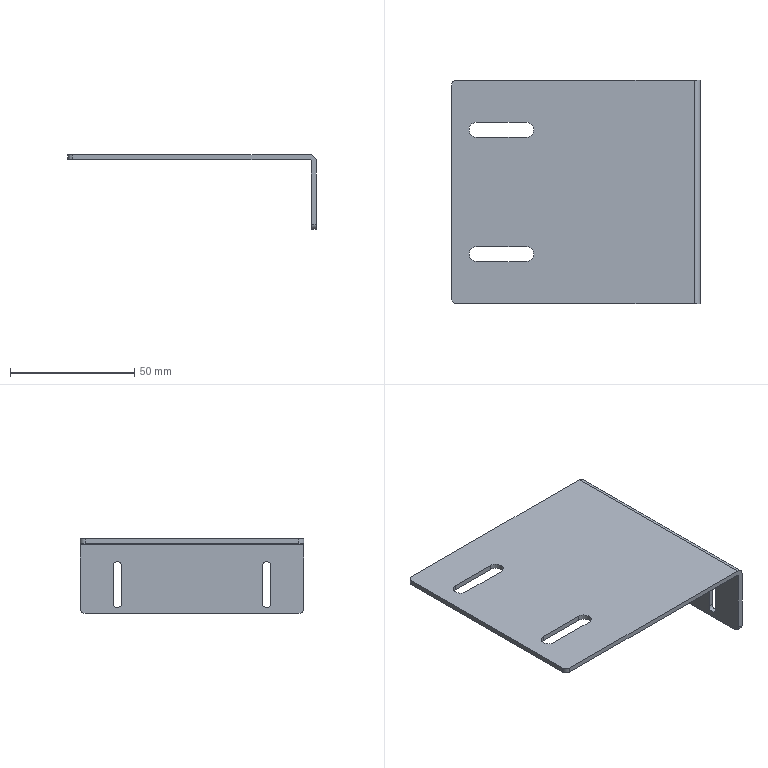Part | SolidWorks | features BaseBody 1 | 1 solid | 34 faces | box 100 x 90 x 30 mm | volume 22076 mm3 | cylinder 18 | plane 16 | commonest cylinder face diameters 3.5 x6 6 x6 4 x4 1 x1 5 x1
STEP:
#1=CARTESIAN_POINT('',(-93.,70.,0.));
#2=VERTEX_POINT('',#1);
#3=CARTESIAN_POINT('',(-90.,73.,0.));
#4=VERTEX_POINT('',#3);
#5=CARTESIAN_POINT('',(-90.,70.,0.));
#6=DIRECTION('',(0.,0.,-1.));
#7=DIRECTION('',(-1.,0.,0.));
#8=AXIS2_PLACEMENT_3D('',#5,#6,#7);
#9=CIRCLE('',#8,3.);
#10=EDGE_CURVE('',#2,#4,#9,.T.);
#11=ORIENTED_EDGE('',*,*,#10,.F.);
#12=CARTESIAN_POINT('',(-93.,70.,-2.));
#13=VERTEX_POINT('',#12);
#14=CARTESIAN_POINT('',(-93.,70.,8.));
#15=DIRECTION('',(0.,0.,-1.));
#16=VECTOR('',#15,1000.);
#17=LINE('',#14,#16);
#18=EDGE_CURVE('',#2,#13,#17,.T.);
#19=ORIENTED_EDGE('',*,*,#18,.T.);
#20=CARTESIAN_POINT('',(-90.,73.,-2.));
#21=VERTEX_POINT('',#20);
#22=CARTESIAN_POINT('',(-90.,70.,-2.));
#23=DIRECTION('',(0.,0.,1.));
#24=DIRECTION('',(-1.,0.,0.));
#25=AXIS2_PLACEMENT_3D('',#22,#23,#24);
#26=CIRCLE('',#25,3.);
#27=EDGE_CURVE('',#21,#13,#26,.T.);
#28=ORIENTED_EDGE('',*,*,#27,.F.);
#29=CARTESIAN_POINT('',(-90.,73.,8.));
#30=DIRECTION('',(0.,0.,1.));
#31=VECTOR('',#30,1000.);
#32=LINE('',#29,#31);
#33=EDGE_CURVE('',#21,#4,#32,.T.);
#34=ORIENTED_EDGE('',*,*,#33,.T.);
#35=EDGE_LOOP('',(#11,#19,#28,#34));
#36=FACE_OUTER_BOUND('',#35,.T.);
#37=CARTESIAN_POINT('',(-90.,70.,8.));
#38=DIRECTION('',(0.,0.,-1.));
#39=DIRECTION('',(-1.,0.,0.));
#40=AXIS2_PLACEMENT_3D('',#37,#38,#39);
#41=CYLINDRICAL_SURFACE('',#40,3.);
#42=ADVANCED_FACE('',(#36),#41,.F.);
#43=CARTESIAN_POINT('',(-93.,20.,0.));
#44=VERTEX_POINT('',#43);
#45=CARTESIAN_POINT('',(-90.,23.,0.));
#46=VERTEX_POINT('',#45);
#47=CARTESIAN_POINT('',(-90.,20.,0.));
#48=DIRECTION('',(0.,0.,-1.));
#49=DIRECTION('',(-1.,0.,0.));
#50=AXIS2_PLACEMENT_3D('',#47,#48,#49);
#51=CIRCLE('',#50,3.);
#52=EDGE_CURVE('',#44,#46,#51,.T.);
#53=ORIENTED_EDGE('',*,*,#52,.F.);
#54=CARTESIAN_POINT('',(-93.,20.,-2.));
#55=VERTEX_POINT('',#54);
#56=CARTESIAN_POINT('',(-93.,20.,8.));
#57=DIRECTION('',(0.,0.,-1.));
#58=VECTOR('',#57,1000.);
#59=LINE('',#56,#58);
#60=EDGE_CURVE('',#44,#55,#59,.T.);
#61=ORIENTED_EDGE('',*,*,#60,.T.);
#62=CARTESIAN_POINT('',(-90.,23.,-2.));
#63=VERTEX_POINT('',#62);
#64=CARTESIAN_POINT('',(-90.,20.,-2.));
#65=DIRECTION('',(0.,0.,1.));
#66=DIRECTION('',(-1.,0.,0.));
#67=AXIS2_PLACEMENT_3D('',#64,#65,#66);
#68=CIRCLE('',#67,3.);
#69=EDGE_CURVE('',#63,#55,#68,.T.);
#70=ORIENTED_EDGE('',*,*,#69,.F.);
#71=CARTESIAN_POINT('',(-90.,23.,8.));
#72=DIRECTION('',(0.,0.,1.));
#73=VECTOR('',#72,1000.);
#74=LINE('',#71,#73);
#75=EDGE_CURVE('',#63,#46,#74,.T.);
#76=ORIENTED_EDGE('',*,*,#75,.T.);
#77=EDGE_LOOP('',(#53,#61,#70,#76));
#78=FACE_OUTER_BOUND('',#77,.T.);
#79=CARTESIAN_POINT('',(-90.,20.,8.));
#80=DIRECTION('',(0.,0.,-1.));
#81=DIRECTION('',(-1.,0.,0.));
#82=AXIS2_PLACEMENT_3D('',#79,#80,#81);
#83=CYLINDRICAL_SURFACE('',#82,3.);
#84=ADVANCED_FACE('',(#78),#83,.F.);
#85=CARTESIAN_POINT('',(0.,75.,-9.25));
#86=VERTEX_POINT('',#85);
#87=CARTESIAN_POINT('',(0.,76.75,-11.));
#88=VERTEX_POINT('',#87);
#89=CARTESIAN_POINT('',(0.,75.,-11.));
#90=DIRECTION('',(-1.,0.,0.));
#91=DIRECTION('',(0.,0.,1.));
#92=AXIS2_PLACEMENT_3D('',#89,#90,#91);
#93=CIRCLE('',#92,1.75);
#94=EDGE_CURVE('',#86,#88,#93,.T.);
#95=ORIENTED_EDGE('',*,*,#94,.F.);
#96=CARTESIAN_POINT('',(-2.,75.,-9.25));
#97=VERTEX_POINT('',#96);
#98=CARTESIAN_POINT('',(8.,75.,-9.25));
#99=DIRECTION('',(-1.,0.,0.));
#100=VECTOR('',#99,1000.);
#101=LINE('',#98,#100);
#102=EDGE_CURVE('',#86,#97,#101,.T.);
#103=ORIENTED_EDGE('',*,*,#102,.T.);
#104=CARTESIAN_POINT('',(-2.,76.75,-11.));
#105=VERTEX_POINT('',#104);
#106=CARTESIAN_POINT('',(-2.,75.,-11.));
#107=DIRECTION('',(1.,0.,0.));
#108=DIRECTION('',(0.,0.,1.));
#109=AXIS2_PLACEMENT_3D('',#106,#107,#108);
#110=CIRCLE('',#109,1.75);
#111=EDGE_CURVE('',#105,#97,#110,.T.);
#112=ORIENTED_EDGE('',*,*,#111,.F.);
#113=CARTESIAN_POINT('',(8.,76.75,-11.));
#114=DIRECTION('',(1.,0.,0.));
#115=VECTOR('',#114,1000.);
#116=LINE('',#113,#115);
#117=EDGE_CURVE('',#105,#88,#116,.T.);
#118=ORIENTED_EDGE('',*,*,#117,.T.);
#119=EDGE_LOOP('',(#95,#103,#112,#118));
#120=FACE_OUTER_BOUND('',#119,.T.);
#121=CARTESIAN_POINT('',(8.,75.,-11.));
#122=DIRECTION('',(-1.,0.,0.));
#123=DIRECTION('',(0.,0.,1.));
#124=AXIS2_PLACEMENT_3D('',#121,#122,#123);
#125=CYLINDRICAL_SURFACE('',#124,1.75);
#126=ADVANCED_FACE('',(#120),#125,.F.);
#127=CARTESIAN_POINT('',(0.,15.,-9.25));
#128=VERTEX_POINT('',#127);
#129=CARTESIAN_POINT('',(0.,16.75,-11.));
#130=VERTEX_POINT('',#129);
#131=CARTESIAN_POINT('',(0.,15.,-11.));
#132=DIRECTION('',(-1.,0.,0.));
#133=DIRECTION('',(0.,0.,1.));
#134=AXIS2_PLACEMENT_3D('',#131,#132,#133);
#135=CIRCLE('',#134,1.75);
#136=EDGE_CURVE('',#128,#130,#135,.T.);
#137=ORIENTED_EDGE('',*,*,#136,.F.);
#138=CARTESIAN_POINT('',(-2.,15.,-9.25));
#139=VERTEX_POINT('',#138);
#140=CARTESIAN_POINT('',(8.,15.,-9.25));
#141=DIRECTION('',(-1.,0.,0.));
#142=VECTOR('',#141,1000.);
#143=LINE('',#140,#142);
#144=EDGE_CURVE('',#128,#139,#143,.T.);
#145=ORIENTED_EDGE('',*,*,#144,.T.);
#146=CARTESIAN_POINT('',(-2.,16.75,-11.));
#147=VERTEX_POINT('',#146);
#148=CARTESIAN_POINT('',(-2.,15.,-11.));
#149=DIRECTION('',(1.,0.,0.));
#150=DIRECTION('',(0.,0.,1.));
#151=AXIS2_PLACEMENT_3D('',#148,#149,#150);
#152=CIRCLE('',#151,1.75);
#153=EDGE_CURVE('',#147,#139,#152,.T.);
#154=ORIENTED_EDGE('',*,*,#153,.F.);
#155=CARTESIAN_POINT('',(8.,16.75,-11.));
#156=DIRECTION('',(1.,0.,0.));
#157=VECTOR('',#156,1000.);
#158=LINE('',#155,#157);
#159=EDGE_CURVE('',#147,#130,#158,.T.);
#160=ORIENTED_EDGE('',*,*,#159,.T.);
#161=EDGE_LOOP('',(#137,#145,#154,#160));
#162=FACE_OUTER_BOUND('',#161,.T.);
#163=CARTESIAN_POINT('',(8.,15.,-11.));
#164=DIRECTION('',(-1.,0.,0.));
#165=DIRECTION('',(0.,0.,1.));
#166=AXIS2_PLACEMENT_3D('',#163,#164,#165);
#167=CYLINDRICAL_SURFACE('',#166,1.75);
#168=ADVANCED_FACE('',(#162),#167,.F.);
#169=CARTESIAN_POINT('',(-2.5,90.,0.));
#170=VERTEX_POINT('',#169);
#171=CARTESIAN_POINT('',(-98.,90.,0.));
#172=VERTEX_POINT('',#171);
#173=CARTESIAN_POINT('',(0.,90.,0.));
#174=DIRECTION('',(-1.,0.,0.));
#175=VECTOR('',#174,1000.);
#176=LINE('',#173,#175);
#177=EDGE_CURVE('',#170,#172,#176,.T.);
#178=ORIENTED_EDGE('',*,*,#177,.T.);
#179=CARTESIAN_POINT('',(-100.,88.,0.));
#180=VERTEX_POINT('',#179);
#181=CARTESIAN_POINT('',(-98.,88.,0.));
#182=DIRECTION('',(0.,0.,1.));
#183=DIRECTION('',(-1.,0.,0.));
#184=AXIS2_PLACEMENT_3D('',#181,#182,#183);
#185=CIRCLE('',#184,2.);
#186=EDGE_CURVE('',#172,#180,#185,.T.);
#187=ORIENTED_EDGE('',*,*,#186,.T.);
#188=CARTESIAN_POINT('',(-100.,2.,0.));
#189=VERTEX_POINT('',#188);
#190=CARTESIAN_POINT('',(-100.,90.,0.));
#191=DIRECTION('',(0.,-1.,0.));
#192=VECTOR('',#191,1000.);
#193=LINE('',#190,#192);
#194=EDGE_CURVE('',#180,#189,#193,.T.);
#195=ORIENTED_EDGE('',*,*,#194,.T.);
#196=CARTESIAN_POINT('',(-98.,0.,0.));
#197=VERTEX_POINT('',#196);
#198=CARTESIAN_POINT('',(-98.,2.,0.));
#199=DIRECTION('',(0.,0.,1.));
#200=DIRECTION('',(1.,0.,0.));
#201=AXIS2_PLACEMENT_3D('',#198,#199,#200);
#202=CIRCLE('',#201,2.);
#203=EDGE_CURVE('',#189,#197,#202,.T.);
#204=ORIENTED_EDGE('',*,*,#203,.T.);
#205=CARTESIAN_POINT('',(-2.5,0.,0.));
#206=VERTEX_POINT('',#205);
#207=CARTESIAN_POINT('',(0.,0.,0.));
#208=DIRECTION('',(1.,0.,0.));
#209=VECTOR('',#208,1000.);
#210=LINE('',#207,#209);
#211=EDGE_CURVE('',#197,#206,#210,.T.);
#212=ORIENTED_EDGE('',*,*,#211,.T.);
#213=CARTESIAN_POINT('',(-2.5,90.,0.));
#214=DIRECTION('',(0.,1.,0.));
#215=VECTOR('',#214,1000.);
#216=LINE('',#213,#215);
#217=EDGE_CURVE('',#206,#170,#216,.T.);
#218=ORIENTED_EDGE('',*,*,#217,.T.);
#219=EDGE_LOOP('',(#178,#187,#195,#204,#212,#218));
#220=FACE_OUTER_BOUND('',#219,.T.);
#221=CARTESIAN_POINT('',(-90.,67.,0.));
#222=VERTEX_POINT('',#221);
#223=CARTESIAN_POINT('',(-90.,70.,0.));
#224=DIRECTION('',(0.,0.,-1.));
#225=DIRECTION('',(-1.,0.,0.));
#226=AXIS2_PLACEMENT_3D('',#223,#224,#225);
#227=CIRCLE('',#226,3.);
#228=EDGE_CURVE('',#222,#2,#227,.T.);
#229=ORIENTED_EDGE('',*,*,#228,.T.);
#230=ORIENTED_EDGE('',*,*,#10,.T.);
#231=CARTESIAN_POINT('',(-70.,73.,0.));
#232=VERTEX_POINT('',#231);
#233=CARTESIAN_POINT('',(0.,73.,0.));
#234=DIRECTION('',(1.,0.,0.));
#235=VECTOR('',#234,1000.);
#236=LINE('',#233,#235);
#237=EDGE_CURVE('',#4,#232,#236,.T.);
#238=ORIENTED_EDGE('',*,*,#237,.T.);
#239=CARTESIAN_POINT('',(-70.,67.,0.));
#240=VERTEX_POINT('',#239);
#241=CARTESIAN_POINT('',(-70.,70.,0.));
#242=DIRECTION('',(0.,0.,-1.));
#243=DIRECTION('',(-1.,0.,0.));
#244=AXIS2_PLACEMENT_3D('',#241,#242,#243);
#245=CIRCLE('',#244,3.);
#246=EDGE_CURVE('',#232,#240,#245,.T.);
#247=ORIENTED_EDGE('',*,*,#246,.T.);
#248=CARTESIAN_POINT('',(0.,67.,0.));
#249=DIRECTION('',(-1.,0.,0.));
#250=VECTOR('',#249,1000.);
#251=LINE('',#248,#250);
#252=EDGE_CURVE('',#240,#222,#251,.T.);
#253=ORIENTED_EDGE('',*,*,#252,.T.);
#254=EDGE_LOOP('',(#229,#230,#238,#247,#253));
#255=FACE_BOUND('',#254,.T.);
#256=CARTESIAN_POINT('',(-90.,17.,0.));
#257=VERTEX_POINT('',#256);
#258=CARTESIAN_POINT('',(-90.,20.,0.));
#259=DIRECTION('',(0.,0.,-1.));
#260=DIRECTION('',(-1.,0.,0.));
#261=AXIS2_PLACEMENT_3D('',#258,#259,#260);
#262=CIRCLE('',#261,3.);
#263=EDGE_CURVE('',#257,#44,#262,.T.);
#264=ORIENTED_EDGE('',*,*,#263,.T.);
#265=ORIENTED_EDGE('',*,*,#52,.T.);
#266=CARTESIAN_POINT('',(-70.,23.,0.));
#267=VERTEX_POINT('',#266);
#268=CARTESIAN_POINT('',(0.,23.,0.));
#269=DIRECTION('',(1.,0.,0.));
#270=VECTOR('',#269,1000.);
#271=LINE('',#268,#270);
#272=EDGE_CURVE('',#46,#267,#271,.T.);
#273=ORIENTED_EDGE('',*,*,#272,.T.);
#274=CARTESIAN_POINT('',(-70.,17.,0.));
#275=VERTEX_POINT('',#274);
#276=CARTESIAN_POINT('',(-70.,20.,0.));
#277=DIRECTION('',(0.,0.,-1.));
#278=DIRECTION('',(-1.,0.,0.));
#279=AXIS2_PLACEMENT_3D('',#276,#277,#278);
#280=CIRCLE('',#279,3.);
#281=EDGE_CURVE('',#267,#275,#280,.T.);
#282=ORIENTED_EDGE('',*,*,#281,.T.);
#283=CARTESIAN_POINT('',(0.,17.,0.));
#284=DIRECTION('',(-1.,0.,0.));
#285=VECTOR('',#284,1000.);
#286=LINE('',#283,#285);
#287=EDGE_CURVE('',#275,#257,#286,.T.);
#288=ORIENTED_EDGE('',*,*,#287,.T.);
#289=EDGE_LOOP('',(#264,#265,#273,#282,#288));
#290=FACE_BOUND('',#289,.T.);
#291=CARTESIAN_POINT('',(0.,90.,0.));
#292=DIRECTION('',(0.,0.,1.));
#293=DIRECTION('',(1.,0.,0.));
#294=AXIS2_PLACEMENT_3D('',#291,#292,#293);
#295=PLANE('',#294);
#296=ADVANCED_FACE('',(#220,#255,#290),#295,.T.);
#297=CARTESIAN_POINT('',(-98.,90.,-2.));
#298=VERTEX_POINT('',#297);
#299=CARTESIAN_POINT('',(-100.,88.,-2.));
#300=VERTEX_POINT('',#299);
#301=CARTESIAN_POINT('',(-98.,88.,-2.));
#302=DIRECTION('',(0.,0.,1.));
#303=DIRECTION('',(-1.,0.,0.));
#304=AXIS2_PLACEMENT_3D('',#301,#302,#303);
#305=CIRCLE('',#304,2.);
#306=EDGE_CURVE('',#298,#300,#305,.T.);
#307=ORIENTED_EDGE('',*,*,#306,.T.);
#308=CARTESIAN_POINT('',(-100.,88.,0.));
#309=DIRECTION('',(0.,0.,1.));
#310=VECTOR('',#309,1000.);
#311=LINE('',#308,#310);
#312=EDGE_CURVE('',#300,#180,#311,.T.);
#313=ORIENTED_EDGE('',*,*,#312,.T.);
#314=ORIENTED_EDGE('',*,*,#186,.F.);
#315=CARTESIAN_POINT('',(-98.,90.,0.));
#316=DIRECTION('',(0.,0.,-1.));
#317=VECTOR('',#316,1000.);
#318=LINE('',#315,#317);
#319=EDGE_CURVE('',#172,#298,#318,.T.);
#320=ORIENTED_EDGE('',*,*,#319,.T.);
#321=EDGE_LOOP('',(#307,#313,#314,#320));
#322=FACE_OUTER_BOUND('',#321,.T.);
#323=CARTESIAN_POINT('',(-98.,88.,0.));
#324=DIRECTION('',(0.,0.,-1.));
#325=DIRECTION('',(-1.,0.,0.));
#326=AXIS2_PLACEMENT_3D('',#323,#324,#325);
#327=CYLINDRICAL_SURFACE('',#326,2.);
#328=ADVANCED_FACE('',(#322),#327,.T.);
#329=ORIENTED_EDGE('',*,*,#177,.F.);
#330=CARTESIAN_POINT('',(0.,90.,-2.5));
#331=VERTEX_POINT('',#330);
#332=CARTESIAN_POINT('',(-2.5,90.,-2.5));
#333=DIRECTION('',(0.,-1.,0.));
#334=DIRECTION('',(0.,0.,-1.));
#335=AXIS2_PLACEMENT_3D('',#332,#333,#334);
#336=CIRCLE('',#335,2.5);
#337=EDGE_CURVE('',#331,#170,#336,.T.);
#338=ORIENTED_EDGE('',*,*,#337,.F.);
#339=CARTESIAN_POINT('',(0.,90.,-28.));
#340=VERTEX_POINT('',#339);
#341=CARTESIAN_POINT('',(0.,90.,-30.));
#342=DIRECTION('',(0.,0.,1.));
#343=VECTOR('',#342,1000.);
#344=LINE('',#341,#343);
#345=EDGE_CURVE('',#340,#331,#344,.T.);
#346=ORIENTED_EDGE('',*,*,#345,.F.);
#347=CARTESIAN_POINT('',(-2.,90.,-28.));
#348=VERTEX_POINT('',#347);
#349=CARTESIAN_POINT('',(-2.5,90.,-28.));
#350=DIRECTION('',(-1.,0.,0.));
#351=VECTOR('',#350,1000.);
#352=LINE('',#349,#351);
#353=EDGE_CURVE('',#340,#348,#352,.T.);
#354=ORIENTED_EDGE('',*,*,#353,.T.);
#355=CARTESIAN_POINT('',(-2.,90.,-2.5));
#356=VERTEX_POINT('',#355);
#357=CARTESIAN_POINT('',(-2.,90.,-2.5));
#358=DIRECTION('',(0.,0.,1.));
#359=VECTOR('',#358,1000.);
#360=LINE('',#357,#359);
#361=EDGE_CURVE('',#348,#356,#360,.T.);
#362=ORIENTED_EDGE('',*,*,#361,.T.);
#363=CARTESIAN_POINT('',(-2.5,90.,-2.));
#364=VERTEX_POINT('',#363);
#365=CARTESIAN_POINT('',(-2.5,90.,-2.5));
#366=DIRECTION('',(0.,-1.,0.));
#367=DIRECTION('',(0.,0.,-1.));
#368=AXIS2_PLACEMENT_3D('',#365,#366,#367);
#369=CIRCLE('',#368,0.5);
#370=EDGE_CURVE('',#356,#364,#369,.T.);
#371=ORIENTED_EDGE('',*,*,#370,.T.);
#372=CARTESIAN_POINT('',(-2.,90.,-2.));
#373=DIRECTION('',(-1.,0.,0.));
#374=VECTOR('',#373,1000.);
#375=LINE('',#372,#374);
#376=EDGE_CURVE('',#364,#298,#375,.T.);
#377=ORIENTED_EDGE('',*,*,#376,.T.);
#378=ORIENTED_EDGE('',*,*,#319,.F.);
#379=EDGE_LOOP('',(#329,#338,#346,#354,#362,#371,#377,#378));
#380=FACE_OUTER_BOUND('',#379,.T.);
#381=CARTESIAN_POINT('',(-2.,90.,-2.5));
#382=DIRECTION('',(0.,1.,0.));
#383=DIRECTION('',(0.,0.,1.));
#384=AXIS2_PLACEMENT_3D('',#381,#382,#383);
#385=PLANE('',#384);
#386=ADVANCED_FACE('',(#380),#385,.T.);
#387=ORIENTED_EDGE('',*,*,#337,.T.);
#388=ORIENTED_EDGE('',*,*,#217,.F.);
#389=CARTESIAN_POINT('',(0.,0.,-2.5));
#390=VERTEX_POINT('',#389);
#391=CARTESIAN_POINT('',(-2.5,0.,-2.5));
#392=DIRECTION('',(0.,1.,0.));
#393=DIRECTION('',(0.,0.,-1.));
#394=AXIS2_PLACEMENT_3D('',#391,#392,#393);
#395=CIRCLE('',#394,2.5);
#396=EDGE_CURVE('',#206,#390,#395,.T.);
#397=ORIENTED_EDGE('',*,*,#396,.T.);
#398=CARTESIAN_POINT('',(0.,90.,-2.5));
#399=DIRECTION('',(0.,1.,0.));
#400=VECTOR('',#399,1000.);
#401=LINE('',#398,#400);
#402=EDGE_CURVE('',#390,#331,#401,.T.);
#403=ORIENTED_EDGE('',*,*,#402,.T.);
#404=EDGE_LOOP('',(#387,#388,#397,#403));
#405=FACE_OUTER_BOUND('',#404,.T.);
#406=CARTESIAN_POINT('',(-2.5,90.,-2.5));
#407=DIRECTION('',(0.,-1.,0.));
#408=DIRECTION('',(0.,0.,-1.));
#409=AXIS2_PLACEMENT_3D('',#406,#407,#408);
#410=CYLINDRICAL_SURFACE('',#409,2.5);
#411=ADVANCED_FACE('',(#405),#410,.T.);
#412=CARTESIAN_POINT('',(-98.,0.,-2.));
#413=VERTEX_POINT('',#412);
#414=CARTESIAN_POINT('',(-98.,0.,-2.5));
#415=DIRECTION('',(0.,0.,1.));
#416=VECTOR('',#415,1000.);
#417=LINE('',#414,#416);
#418=EDGE_CURVE('',#413,#197,#417,.T.);
#419=ORIENTED_EDGE('',*,*,#418,.F.);
#420=CARTESIAN_POINT('',(-2.5,0.,-2.));
#421=VERTEX_POINT('',#420);
#422=CARTESIAN_POINT('',(-2.5,0.,-2.));
#423=DIRECTION('',(-1.,0.,0.));
#424=VECTOR('',#423,1000.);
#425=LINE('',#422,#424);
#426=EDGE_CURVE('',#421,#413,#425,.T.);
#427=ORIENTED_EDGE('',*,*,#426,.F.);
#428=CARTESIAN_POINT('',(-2.,0.,-2.5));
#429=VERTEX_POINT('',#428);
#430=CARTESIAN_POINT('',(-2.5,0.,-2.5));
#431=DIRECTION('',(0.,1.,0.));
#432=DIRECTION('',(0.,0.,-1.));
#433=AXIS2_PLACEMENT_3D('',#430,#431,#432);
#434=CIRCLE('',#433,0.5);
#435=EDGE_CURVE('',#421,#429,#434,.T.);
#436=ORIENTED_EDGE('',*,*,#435,.T.);
#437=CARTESIAN_POINT('',(-2.,0.,-28.));
#438=VERTEX_POINT('',#437);
#439=CARTESIAN_POINT('',(-2.,0.,-2.));
#440=DIRECTION('',(0.,0.,-1.));
#441=VECTOR('',#440,1000.);
#442=LINE('',#439,#441);
#443=EDGE_CURVE('',#429,#438,#442,.T.);
#444=ORIENTED_EDGE('',*,*,#443,.T.);
#445=CARTESIAN_POINT('',(0.,0.,-28.));
#446=VERTEX_POINT('',#445);
#447=CARTESIAN_POINT('',(-2.5,0.,-28.));
#448=DIRECTION('',(-1.,0.,0.));
#449=VECTOR('',#448,1000.);
#450=LINE('',#447,#449);
#451=EDGE_CURVE('',#446,#438,#450,.T.);
#452=ORIENTED_EDGE('',*,*,#451,.F.);
#453=CARTESIAN_POINT('',(0.,0.,-30.));
#454=DIRECTION('',(0.,0.,-1.));
#455=VECTOR('',#454,1000.);
#456=LINE('',#453,#455);
#457=EDGE_CURVE('',#390,#446,#456,.T.);
#458=ORIENTED_EDGE('',*,*,#457,.F.);
#459=ORIENTED_EDGE('',*,*,#396,.F.);
#460=ORIENTED_EDGE('',*,*,#211,.F.);
#461=EDGE_LOOP('',(#419,#427,#436,#444,#452,#458,#459,#460));
#462=FACE_OUTER_BOUND('',#461,.T.);
#463=CARTESIAN_POINT('',(-2.5,0.,-2.5));
#464=DIRECTION('',(0.,1.,0.));
#465=DIRECTION('',(0.,0.,1.));
#466=AXIS2_PLACEMENT_3D('',#463,#464,#465);
#467=PLANE('',#466);
#468=ADVANCED_FACE('',(#462),#467,.F.);
#469=CARTESIAN_POINT('',(-100.,2.,-2.));
#470=VERTEX_POINT('',#469);
#471=CARTESIAN_POINT('',(-98.,2.,-2.));
#472=DIRECTION('',(0.,0.,1.));
#473=DIRECTION('',(1.,0.,0.));
#474=AXIS2_PLACEMENT_3D('',#471,#472,#473);
#475=CIRCLE('',#474,2.);
#476=EDGE_CURVE('',#470,#413,#475,.T.);
#477=ORIENTED_EDGE('',*,*,#476,.T.);
#478=ORIENTED_EDGE('',*,*,#418,.T.);
#479=ORIENTED_EDGE('',*,*,#203,.F.);
#480=CARTESIAN_POINT('',(-100.,2.,-2.5));
#481=DIRECTION('',(0.,0.,-1.));
#482=VECTOR('',#481,1000.);
#483=LINE('',#480,#482);
#484=EDGE_CURVE('',#189,#470,#483,.T.);
#485=ORIENTED_EDGE('',*,*,#484,.T.);
#486=EDGE_LOOP('',(#477,#478,#479,#485));
#487=FACE_OUTER_BOUND('',#486,.T.);
#488=CARTESIAN_POINT('',(-98.,2.,-2.5));
#489=DIRECTION('',(0.,0.,1.));
#490=DIRECTION('',(1.,0.,0.));
#491=AXIS2_PLACEMENT_3D('',#488,#489,#490);
#492=CYLINDRICAL_SURFACE('',#491,2.);
#493=ADVANCED_FACE('',(#487),#492,.T.);
#494=ORIENTED_EDGE('',*,*,#194,.F.);
#495=ORIENTED_EDGE('',*,*,#312,.F.);
#496=CARTESIAN_POINT('',(-100.,90.,-2.));
#497=DIRECTION('',(0.,-1.,0.));
#498=VECTOR('',#497,1000.);
#499=LINE('',#496,#498);
#500=EDGE_CURVE('',#300,#470,#499,.T.);
#501=ORIENTED_EDGE('',*,*,#500,.T.);
#502=ORIENTED_EDGE('',*,*,#484,.F.);
#503=EDGE_LOOP('',(#494,#495,#501,#502));
#504=FACE_OUTER_BOUND('',#503,.T.);
#505=CARTESIAN_POINT('',(-100.,90.,0.));
#506=DIRECTION('',(-1.,0.,0.));
#507=DIRECTION('',(0.,0.,1.));
#508=AXIS2_PLACEMENT_3D('',#505,#506,#507);
#509=PLANE('',#508);
#510=ADVANCED_FACE('',(#504),#509,.T.);
#511=ORIENTED_EDGE('',*,*,#33,.F.);
#512=CARTESIAN_POINT('',(-70.,73.,-2.));
#513=VERTEX_POINT('',#512);
#514=CARTESIAN_POINT('',(-70.,73.,-2.));
#515=DIRECTION('',(-1.,0.,0.));
#516=VECTOR('',#515,1000.);
#517=LINE('',#514,#516);
#518=EDGE_CURVE('',#513,#21,#517,.T.);
#519=ORIENTED_EDGE('',*,*,#518,.F.);
#520=CARTESIAN_POINT('',(-70.,73.,8.));
#521=DIRECTION('',(0.,0.,-1.));
#522=VECTOR('',#521,1000.);
#523=LINE('',#520,#522);
#524=EDGE_CURVE('',#232,#513,#523,.T.);
#525=ORIENTED_EDGE('',*,*,#524,.F.);
#526=ORIENTED_EDGE('',*,*,#237,.F.);
#527=EDGE_LOOP('',(#511,#519,#525,#526));
#528=FACE_OUTER_BOUND('',#527,.T.);
#529=CARTESIAN_POINT('',(-70.,73.,8.));
#530=DIRECTION('',(0.,1.,0.));
#531=DIRECTION('',(0.,0.,1.));
#532=AXIS2_PLACEMENT_3D('',#529,#530,#531);
#533=PLANE('',#532);
#534=ADVANCED_FACE('',(#528),#533,.F.);
#535=ORIENTED_EDGE('',*,*,#18,.F.);
#536=ORIENTED_EDGE('',*,*,#228,.F.);
#537=CARTESIAN_POINT('',(-90.,67.,-2.));
#538=VERTEX_POINT('',#537);
#539=CARTESIAN_POINT('',(-90.,67.,8.));
#540=DIRECTION('',(0.,0.,1.));
#541=VECTOR('',#540,1000.);
#542=LINE('',#539,#541);
#543=EDGE_CURVE('',#538,#222,#542,.T.);
#544=ORIENTED_EDGE('',*,*,#543,.F.);
#545=CARTESIAN_POINT('',(-90.,70.,-2.));
#546=DIRECTION('',(0.,0.,1.));
#547=DIRECTION('',(-1.,0.,0.));
#548=AXIS2_PLACEMENT_3D('',#545,#546,#547);
#549=CIRCLE('',#548,3.);
#550=EDGE_CURVE('',#13,#538,#549,.T.);
#551=ORIENTED_EDGE('',*,*,#550,.F.);
#552=EDGE_LOOP('',(#535,#536,#544,#551));
#553=FACE_OUTER_BOUND('',#552,.T.);
#554=CARTESIAN_POINT('',(-90.,70.,8.));
#555=DIRECTION('',(0.,0.,-1.));
#556=DIRECTION('',(-1.,0.,0.));
#557=AXIS2_PLACEMENT_3D('',#554,#555,#556);
#558=CYLINDRICAL_SURFACE('',#557,3.);
#559=ADVANCED_FACE('',(#553),#558,.F.);
#560=CARTESIAN_POINT('',(-70.,67.,-2.));
#561=VERTEX_POINT('',#560);
#562=CARTESIAN_POINT('',(-70.,67.,8.));
#563=DIRECTION('',(0.,0.,1.));
#564=VECTOR('',#563,1000.);
#565=LINE('',#562,#564);
#566=EDGE_CURVE('',#561,#240,#565,.T.);
#567=ORIENTED_EDGE('',*,*,#566,.F.);
#568=CARTESIAN_POINT('',(-70.,67.,-2.));
#569=DIRECTION('',(1.,0.,0.));
#570=VECTOR('',#569,1000.);
#571=LINE('',#568,#570);
#572=EDGE_CURVE('',#538,#561,#571,.T.);
#573=ORIENTED_EDGE('',*,*,#572,.F.);
#574=ORIENTED_EDGE('',*,*,#543,.T.);
#575=ORIENTED_EDGE('',*,*,#252,.F.);
#576=EDGE_LOOP('',(#567,#573,#574,#575));
#577=FACE_OUTER_BOUND('',#576,.T.);
#578=CARTESIAN_POINT('',(-70.,67.,8.));
#579=DIRECTION('',(0.,-1.,0.));
#580=DIRECTION('',(0.,0.,-1.));
#581=AXIS2_PLACEMENT_3D('',#578,#579,#580);
#582=PLANE('',#581);
#583=ADVANCED_FACE('',(#577),#582,.F.);
#584=ORIENTED_EDGE('',*,*,#524,.T.);
#585=CARTESIAN_POINT('',(-70.,70.,-2.));
#586=DIRECTION('',(0.,0.,1.));
#587=DIRECTION('',(-1.,0.,0.));
#588=AXIS2_PLACEMENT_3D('',#585,#586,#587);
#589=CIRCLE('',#588,3.);
#590=EDGE_CURVE('',#561,#513,#589,.T.);
#591=ORIENTED_EDGE('',*,*,#590,.F.);
#592=ORIENTED_EDGE('',*,*,#566,.T.);
#593=ORIENTED_EDGE('',*,*,#246,.F.);
#594=EDGE_LOOP('',(#584,#591,#592,#593));
#595=FACE_OUTER_BOUND('',#594,.T.);
#596=CARTESIAN_POINT('',(-70.,70.,8.));
#597=DIRECTION('',(0.,0.,-1.));
#598=DIRECTION('',(-1.,0.,0.));
#599=AXIS2_PLACEMENT_3D('',#596,#597,#598);
#600=CYLINDRICAL_SURFACE('',#599,3.);
#601=ADVANCED_FACE('',(#595),#600,.F.);
#602=ORIENTED_EDGE('',*,*,#75,.F.);
#603=CARTESIAN_POINT('',(-70.,23.,-2.));
#604=VERTEX_POINT('',#603);
#605=CARTESIAN_POINT('',(-70.,23.,-2.));
#606=DIRECTION('',(-1.,0.,0.));
#607=VECTOR('',#606,1000.);
#608=LINE('',#605,#607);
#609=EDGE_CURVE('',#604,#63,#608,.T.);
#610=ORIENTED_EDGE('',*,*,#609,.F.);
#611=CARTESIAN_POINT('',(-70.,23.,8.));
#612=DIRECTION('',(0.,0.,-1.));
#613=VECTOR('',#612,1000.);
#614=LINE('',#611,#613);
#615=EDGE_CURVE('',#267,#604,#614,.T.);
#616=ORIENTED_EDGE('',*,*,#615,.F.);
#617=ORIENTED_EDGE('',*,*,#272,.F.);
#618=EDGE_LOOP('',(#602,#610,#616,#617));
#619=FACE_OUTER_BOUND('',#618,.T.);
#620=CARTESIAN_POINT('',(-70.,23.,8.));
#621=DIRECTION('',(0.,1.,0.));
#622=DIRECTION('',(0.,0.,1.));
#623=AXIS2_PLACEMENT_3D('',#620,#621,#622);
#624=PLANE('',#623);
#625=ADVANCED_FACE('',(#619),#624,.F.);
#626=ORIENTED_EDGE('',*,*,#60,.F.);
#627=ORIENTED_EDGE('',*,*,#263,.F.);
#628=CARTESIAN_POINT('',(-90.,17.,-2.));
#629=VERTEX_POINT('',#628);
#630=CARTESIAN_POINT('',(-90.,17.,8.));
#631=DIRECTION('',(0.,0.,1.));
#632=VECTOR('',#631,1000.);
#633=LINE('',#630,#632);
#634=EDGE_CURVE('',#629,#257,#633,.T.);
#635=ORIENTED_EDGE('',*,*,#634,.F.);
#636=CARTESIAN_POINT('',(-90.,20.,-2.));
#637=DIRECTION('',(0.,0.,1.));
#638=DIRECTION('',(-1.,0.,0.));
#639=AXIS2_PLACEMENT_3D('',#636,#637,#638);
#640=CIRCLE('',#639,3.);
#641=EDGE_CURVE('',#55,#629,#640,.T.);
#642=ORIENTED_EDGE('',*,*,#641,.F.);
#643=EDGE_LOOP('',(#626,#627,#635,#642));
#644=FACE_OUTER_BOUND('',#643,.T.);
#645=CARTESIAN_POINT('',(-90.,20.,8.));
#646=DIRECTION('',(0.,0.,-1.));
#647=DIRECTION('',(-1.,0.,0.));
#648=AXIS2_PLACEMENT_3D('',#645,#646,#647);
#649=CYLINDRICAL_SURFACE('',#648,3.);
#650=ADVANCED_FACE('',(#644),#649,.F.);
#651=CARTESIAN_POINT('',(-70.,17.,-2.));
#652=VERTEX_POINT('',#651);
#653=CARTESIAN_POINT('',(-70.,17.,8.));
#654=DIRECTION('',(0.,0.,1.));
#655=VECTOR('',#654,1000.);
#656=LINE('',#653,#655);
#657=EDGE_CURVE('',#652,#275,#656,.T.);
#658=ORIENTED_EDGE('',*,*,#657,.F.);
#659=CARTESIAN_POINT('',(-70.,17.,-2.));
#660=DIRECTION('',(1.,0.,0.));
#661=VECTOR('',#660,1000.);
#662=LINE('',#659,#661);
#663=EDGE_CURVE('',#629,#652,#662,.T.);
#664=ORIENTED_EDGE('',*,*,#663,.F.);
#665=ORIENTED_EDGE('',*,*,#634,.T.);
#666=ORIENTED_EDGE('',*,*,#287,.F.);
#667=EDGE_LOOP('',(#658,#664,#665,#666));
#668=FACE_OUTER_BOUND('',#667,.T.);
#669=CARTESIAN_POINT('',(-70.,17.,8.));
#670=DIRECTION('',(0.,-1.,0.));
#671=DIRECTION('',(0.,0.,-1.));
#672=AXIS2_PLACEMENT_3D('',#669,#670,#671);
#673=PLANE('',#672);
#674=ADVANCED_FACE('',(#668),#673,.F.);
#675=ORIENTED_EDGE('',*,*,#615,.T.);
#676=CARTESIAN_POINT('',(-70.,20.,-2.));
#677=DIRECTION('',(0.,0.,1.));
#678=DIRECTION('',(-1.,0.,0.));
#679=AXIS2_PLACEMENT_3D('',#676,#677,#678);
#680=CIRCLE('',#679,3.);
#681=EDGE_CURVE('',#652,#604,#680,.T.);
#682=ORIENTED_EDGE('',*,*,#681,.F.);
#683=ORIENTED_EDGE('',*,*,#657,.T.);
#684=ORIENTED_EDGE('',*,*,#281,.F.);
#685=EDGE_LOOP('',(#675,#682,#683,#684));
#686=FACE_OUTER_BOUND('',#685,.T.);
#687=CARTESIAN_POINT('',(-70.,20.,8.));
#688=DIRECTION('',(0.,0.,-1.));
#689=DIRECTION('',(-1.,0.,0.));
#690=AXIS2_PLACEMENT_3D('',#687,#688,#689);
#691=CYLINDRICAL_SURFACE('',#690,3.);
#692=ADVANCED_FACE('',(#686),#691,.F.);
#693=ORIENTED_EDGE('',*,*,#476,.F.);
#694=ORIENTED_EDGE('',*,*,#500,.F.);
#695=ORIENTED_EDGE('',*,*,#306,.F.);
#696=ORIENTED_EDGE('',*,*,#376,.F.);
#697=CARTESIAN_POINT('',(-2.5,90.,-2.));
#698=DIRECTION('',(0.,1.,0.));
#699=VECTOR('',#698,1000.);
#700=LINE('',#697,#699);
#701=EDGE_CURVE('',#421,#364,#700,.T.);
#702=ORIENTED_EDGE('',*,*,#701,.F.);
#703=ORIENTED_EDGE('',*,*,#426,.T.);
#704=EDGE_LOOP('',(#693,#694,#695,#696,#702,#703));
#705=FACE_OUTER_BOUND('',#704,.T.);
#706=ORIENTED_EDGE('',*,*,#590,.T.);
#707=ORIENTED_EDGE('',*,*,#518,.T.);
#708=ORIENTED_EDGE('',*,*,#27,.T.);
#709=ORIENTED_EDGE('',*,*,#550,.T.);
#710=ORIENTED_EDGE('',*,*,#572,.T.);
#711=EDGE_LOOP('',(#706,#707,#708,#709,#710));
#712=FACE_BOUND('',#711,.T.);
#713=ORIENTED_EDGE('',*,*,#681,.T.);
#714=ORIENTED_EDGE('',*,*,#609,.T.);
#715=ORIENTED_EDGE('',*,*,#69,.T.);
#716=ORIENTED_EDGE('',*,*,#641,.T.);
#717=ORIENTED_EDGE('',*,*,#663,.T.);
#718=EDGE_LOOP('',(#713,#714,#715,#716,#717));
#719=FACE_BOUND('',#718,.T.);
#720=CARTESIAN_POINT('',(0.,90.,-2.));
#721=DIRECTION('',(0.,0.,1.));
#722=DIRECTION('',(1.,0.,0.));
#723=AXIS2_PLACEMENT_3D('',#720,#721,#722);
#724=PLANE('',#723);
#725=ADVANCED_FACE('',(#705,#712,#719),#724,.F.);
#726=ORIENTED_EDGE('',*,*,#457,.T.);
#727=CARTESIAN_POINT('',(0.,2.,-30.));
#728=VERTEX_POINT('',#727);
#729=CARTESIAN_POINT('',(0.,2.,-28.));
#730=DIRECTION('',(1.,0.,0.));
#731=DIRECTION('',(0.,0.,-1.));
#732=AXIS2_PLACEMENT_3D('',#729,#730,#731);
#733=CIRCLE('',#732,2.);
#734=EDGE_CURVE('',#446,#728,#733,.T.);
#735=ORIENTED_EDGE('',*,*,#734,.T.);
#736=CARTESIAN_POINT('',(0.,88.,-30.));
#737=VERTEX_POINT('',#736);
#738=CARTESIAN_POINT('',(0.,90.,-30.));
#739=DIRECTION('',(0.,1.,0.));
#740=VECTOR('',#739,1000.);
#741=LINE('',#738,#740);
#742=EDGE_CURVE('',#728,#737,#741,.T.);
#743=ORIENTED_EDGE('',*,*,#742,.T.);
#744=CARTESIAN_POINT('',(0.,88.,-28.));
#745=DIRECTION('',(1.,0.,0.));
#746=DIRECTION('',(0.,0.,-1.));
#747=AXIS2_PLACEMENT_3D('',#744,#745,#746);
#748=CIRCLE('',#747,2.);
#749=EDGE_CURVE('',#737,#340,#748,.T.);
#750=ORIENTED_EDGE('',*,*,#749,.T.);
#751=ORIENTED_EDGE('',*,*,#345,.T.);
#752=ORIENTED_EDGE('',*,*,#402,.F.);
#753=EDGE_LOOP('',(#726,#735,#743,#750,#751,#752));
#754=FACE_OUTER_BOUND('',#753,.T.);
#755=CARTESIAN_POINT('',(0.,73.25,-11.));
#756=VERTEX_POINT('',#755);
#757=CARTESIAN_POINT('',(0.,75.,-11.));
#758=DIRECTION('',(-1.,0.,0.));
#759=DIRECTION('',(0.,0.,1.));
#760=AXIS2_PLACEMENT_3D('',#757,#758,#759);
#761=CIRCLE('',#760,1.75);
#762=EDGE_CURVE('',#756,#86,#761,.T.);
#763=ORIENTED_EDGE('',*,*,#762,.T.);
#764=ORIENTED_EDGE('',*,*,#94,.T.);
#765=CARTESIAN_POINT('',(0.,76.75,-26.));
#766=VERTEX_POINT('',#765);
#767=CARTESIAN_POINT('',(0.,76.75,-30.));
#768=DIRECTION('',(0.,0.,-1.));
#769=VECTOR('',#768,1000.);
#770=LINE('',#767,#769);
#771=EDGE_CURVE('',#88,#766,#770,.T.);
#772=ORIENTED_EDGE('',*,*,#771,.T.);
#773=CARTESIAN_POINT('',(0.,73.25,-26.));
#774=VERTEX_POINT('',#773);
#775=CARTESIAN_POINT('',(0.,75.,-26.));
#776=DIRECTION('',(-1.,0.,0.));
#777=DIRECTION('',(0.,0.,1.));
#778=AXIS2_PLACEMENT_3D('',#775,#776,#777);
#779=CIRCLE('',#778,1.75);
#780=EDGE_CURVE('',#766,#774,#779,.T.);
#781=ORIENTED_EDGE('',*,*,#780,.T.);
#782=CARTESIAN_POINT('',(0.,73.25,-30.));
#783=DIRECTION('',(0.,0.,1.));
#784=VECTOR('',#783,1000.);
#785=LINE('',#782,#784);
#786=EDGE_CURVE('',#774,#756,#785,.T.);
#787=ORIENTED_EDGE('',*,*,#786,.T.);
#788=EDGE_LOOP('',(#763,#764,#772,#781,#787));
#789=FACE_BOUND('',#788,.T.);
#790=CARTESIAN_POINT('',(0.,13.25,-11.));
#791=VERTEX_POINT('',#790);
#792=CARTESIAN_POINT('',(0.,15.,-11.));
#793=DIRECTION('',(-1.,0.,0.));
#794=DIRECTION('',(0.,0.,1.));
#795=AXIS2_PLACEMENT_3D('',#792,#793,#794);
#796=CIRCLE('',#795,1.75);
#797=EDGE_CURVE('',#791,#128,#796,.T.);
#798=ORIENTED_EDGE('',*,*,#797,.T.);
#799=ORIENTED_EDGE('',*,*,#136,.T.);
#800=CARTESIAN_POINT('',(0.,16.75,-26.));
#801=VERTEX_POINT('',#800);
#802=CARTESIAN_POINT('',(0.,16.75,-30.));
#803=DIRECTION('',(0.,0.,-1.));
#804=VECTOR('',#803,1000.);
#805=LINE('',#802,#804);
#806=EDGE_CURVE('',#130,#801,#805,.T.);
#807=ORIENTED_EDGE('',*,*,#806,.T.);
#808=CARTESIAN_POINT('',(0.,13.25,-26.));
#809=VERTEX_POINT('',#808);
#810=CARTESIAN_POINT('',(0.,15.,-26.));
#811=DIRECTION('',(-1.,0.,0.));
#812=DIRECTION('',(0.,0.,1.));
#813=AXIS2_PLACEMENT_3D('',#810,#811,#812);
#814=CIRCLE('',#813,1.75);
#815=EDGE_CURVE('',#801,#809,#814,.T.);
#816=ORIENTED_EDGE('',*,*,#815,.T.);
#817=CARTESIAN_POINT('',(0.,13.25,-30.));
#818=DIRECTION('',(0.,0.,1.));
#819=VECTOR('',#818,1000.);
#820=LINE('',#817,#819);
#821=EDGE_CURVE('',#809,#791,#820,.T.);
#822=ORIENTED_EDGE('',*,*,#821,.T.);
#823=EDGE_LOOP('',(#798,#799,#807,#816,#822));
#824=FACE_BOUND('',#823,.T.);
#825=CARTESIAN_POINT('',(0.,90.,-30.));
#826=DIRECTION('',(1.,0.,0.));
#827=DIRECTION('',(0.,0.,-1.));
#828=AXIS2_PLACEMENT_3D('',#825,#826,#827);
#829=PLANE('',#828);
#830=ADVANCED_FACE('',(#754,#789,#824),#829,.T.);
#831=ORIENTED_EDGE('',*,*,#701,.T.);
#832=ORIENTED_EDGE('',*,*,#370,.F.);
#833=CARTESIAN_POINT('',(-2.,90.,-2.5));
#834=DIRECTION('',(0.,1.,0.));
#835=VECTOR('',#834,1000.);
#836=LINE('',#833,#835);
#837=EDGE_CURVE('',#429,#356,#836,.T.);
#838=ORIENTED_EDGE('',*,*,#837,.F.);
#839=ORIENTED_EDGE('',*,*,#435,.F.);
#840=EDGE_LOOP('',(#831,#832,#838,#839));
#841=FACE_OUTER_BOUND('',#840,.T.);
#842=CARTESIAN_POINT('',(-2.5,90.,-2.5));
#843=DIRECTION('',(0.,-1.,0.));
#844=DIRECTION('',(0.,0.,-1.));
#845=AXIS2_PLACEMENT_3D('',#842,#843,#844);
#846=CYLINDRICAL_SURFACE('',#845,0.5);
#847=ADVANCED_FACE('',(#841),#846,.F.);
#848=ORIENTED_EDGE('',*,*,#734,.F.);
#849=ORIENTED_EDGE('',*,*,#451,.T.);
#850=CARTESIAN_POINT('',(-2.,2.,-30.));
#851=VERTEX_POINT('',#850);
#852=CARTESIAN_POINT('',(-2.,2.,-28.));
#853=DIRECTION('',(1.,0.,0.));
#854=DIRECTION('',(0.,0.,-1.));
#855=AXIS2_PLACEMENT_3D('',#852,#853,#854);
#856=CIRCLE('',#855,2.);
#857=EDGE_CURVE('',#438,#851,#856,.T.);
#858=ORIENTED_EDGE('',*,*,#857,.T.);
#859=CARTESIAN_POINT('',(-2.5,2.,-30.));
#860=DIRECTION('',(1.,0.,0.));
#861=VECTOR('',#860,1000.);
#862=LINE('',#859,#861);
#863=EDGE_CURVE('',#851,#728,#862,.T.);
#864=ORIENTED_EDGE('',*,*,#863,.T.);
#865=EDGE_LOOP('',(#848,#849,#858,#864));
#866=FACE_OUTER_BOUND('',#865,.T.);
#867=CARTESIAN_POINT('',(-2.5,2.,-28.));
#868=DIRECTION('',(1.,0.,0.));
#869=DIRECTION('',(0.,0.,-1.));
#870=AXIS2_PLACEMENT_3D('',#867,#868,#869);
#871=CYLINDRICAL_SURFACE('',#870,2.);
#872=ADVANCED_FACE('',(#866),#871,.T.);
#873=ORIENTED_EDGE('',*,*,#749,.F.);
#874=CARTESIAN_POINT('',(-2.,88.,-30.));
#875=VERTEX_POINT('',#874);
#876=CARTESIAN_POINT('',(-2.,88.,-30.));
#877=DIRECTION('',(-1.,0.,0.));
#878=VECTOR('',#877,1000.);
#879=LINE('',#876,#878);
#880=EDGE_CURVE('',#737,#875,#879,.T.);
#881=ORIENTED_EDGE('',*,*,#880,.T.);
#882=CARTESIAN_POINT('',(-2.,88.,-28.));
#883=DIRECTION('',(1.,0.,0.));
#884=DIRECTION('',(0.,0.,-1.));
#885=AXIS2_PLACEMENT_3D('',#882,#883,#884);
#886=CIRCLE('',#885,2.);
#887=EDGE_CURVE('',#875,#348,#886,.T.);
#888=ORIENTED_EDGE('',*,*,#887,.T.);
#889=ORIENTED_EDGE('',*,*,#353,.F.);
#890=EDGE_LOOP('',(#873,#881,#888,#889));
#891=FACE_OUTER_BOUND('',#890,.T.);
#892=CARTESIAN_POINT('',(-2.,88.,-28.));
#893=DIRECTION('',(1.,0.,0.));
#894=DIRECTION('',(0.,0.,-1.));
#895=AXIS2_PLACEMENT_3D('',#892,#893,#894);
#896=CYLINDRICAL_SURFACE('',#895,2.);
#897=ADVANCED_FACE('',(#891),#896,.T.);
#898=ORIENTED_EDGE('',*,*,#742,.F.);
#899=ORIENTED_EDGE('',*,*,#863,.F.);
#900=CARTESIAN_POINT('',(-2.,90.,-30.));
#901=DIRECTION('',(0.,1.,0.));
#902=VECTOR('',#901,1000.);
#903=LINE('',#900,#902);
#904=EDGE_CURVE('',#851,#875,#903,.T.);
#905=ORIENTED_EDGE('',*,*,#904,.T.);
#906=ORIENTED_EDGE('',*,*,#880,.F.);
#907=EDGE_LOOP('',(#898,#899,#905,#906));
#908=FACE_OUTER_BOUND('',#907,.T.);
#909=CARTESIAN_POINT('',(-2.,90.,-30.));
#910=DIRECTION('',(0.,0.,-1.));
#911=DIRECTION('',(-1.,0.,0.));
#912=AXIS2_PLACEMENT_3D('',#909,#910,#911);
#913=PLANE('',#912);
#914=ADVANCED_FACE('',(#908),#913,.T.);
#915=ORIENTED_EDGE('',*,*,#117,.F.);
#916=CARTESIAN_POINT('',(-2.,76.75,-26.));
#917=VERTEX_POINT('',#916);
#918=CARTESIAN_POINT('',(-2.,76.75,-26.));
#919=DIRECTION('',(0.,0.,1.));
#920=VECTOR('',#919,1000.);
#921=LINE('',#918,#920);
#922=EDGE_CURVE('',#917,#105,#921,.T.);
#923=ORIENTED_EDGE('',*,*,#922,.F.);
#924=CARTESIAN_POINT('',(8.,76.75,-26.));
#925=DIRECTION('',(-1.,0.,0.));
#926=VECTOR('',#925,1000.);
#927=LINE('',#924,#926);
#928=EDGE_CURVE('',#766,#917,#927,.T.);
#929=ORIENTED_EDGE('',*,*,#928,.F.);
#930=ORIENTED_EDGE('',*,*,#771,.F.);
#931=EDGE_LOOP('',(#915,#923,#929,#930));
#932=FACE_OUTER_BOUND('',#931,.T.);
#933=CARTESIAN_POINT('',(8.,76.75,-26.));
#934=DIRECTION('',(0.,1.,0.));
#935=DIRECTION('',(0.,0.,1.));
#936=AXIS2_PLACEMENT_3D('',#933,#934,#935);
#937=PLANE('',#936);
#938=ADVANCED_FACE('',(#932),#937,.F.);
#939=ORIENTED_EDGE('',*,*,#102,.F.);
#940=ORIENTED_EDGE('',*,*,#762,.F.);
#941=CARTESIAN_POINT('',(-2.,73.25,-11.));
#942=VERTEX_POINT('',#941);
#943=CARTESIAN_POINT('',(8.,73.25,-11.));
#944=DIRECTION('',(1.,0.,0.));
#945=VECTOR('',#944,1000.);
#946=LINE('',#943,#945);
#947=EDGE_CURVE('',#942,#756,#946,.T.);
#948=ORIENTED_EDGE('',*,*,#947,.F.);
#949=CARTESIAN_POINT('',(-2.,75.,-11.));
#950=DIRECTION('',(1.,0.,0.));
#951=DIRECTION('',(0.,0.,1.));
#952=AXIS2_PLACEMENT_3D('',#949,#950,#951);
#953=CIRCLE('',#952,1.75);
#954=EDGE_CURVE('',#97,#942,#953,.T.);
#955=ORIENTED_EDGE('',*,*,#954,.F.);
#956=EDGE_LOOP('',(#939,#940,#948,#955));
#957=FACE_OUTER_BOUND('',#956,.T.);
#958=CARTESIAN_POINT('',(8.,75.,-11.));
#959=DIRECTION('',(-1.,0.,0.));
#960=DIRECTION('',(0.,0.,1.));
#961=AXIS2_PLACEMENT_3D('',#958,#959,#960);
#962=CYLINDRICAL_SURFACE('',#961,1.75);
#963=ADVANCED_FACE('',(#957),#962,.F.);
#964=CARTESIAN_POINT('',(-2.,73.25,-26.));
#965=VERTEX_POINT('',#964);
#966=CARTESIAN_POINT('',(8.,73.25,-26.));
#967=DIRECTION('',(1.,0.,0.));
#968=VECTOR('',#967,1000.);
#969=LINE('',#966,#968);
#970=EDGE_CURVE('',#965,#774,#969,.T.);
#971=ORIENTED_EDGE('',*,*,#970,.F.);
#972=CARTESIAN_POINT('',(-2.,73.25,-26.));
#973=DIRECTION('',(0.,0.,-1.));
#974=VECTOR('',#973,1000.);
#975=LINE('',#972,#974);
#976=EDGE_CURVE('',#942,#965,#975,.T.);
#977=ORIENTED_EDGE('',*,*,#976,.F.);
#978=ORIENTED_EDGE('',*,*,#947,.T.);
#979=ORIENTED_EDGE('',*,*,#786,.F.);
#980=EDGE_LOOP('',(#971,#977,#978,#979));
#981=FACE_OUTER_BOUND('',#980,.T.);
#982=CARTESIAN_POINT('',(8.,73.25,-26.));
#983=DIRECTION('',(0.,-1.,0.));
#984=DIRECTION('',(0.,0.,-1.));
#985=AXIS2_PLACEMENT_3D('',#982,#983,#984);
#986=PLANE('',#985);
#987=ADVANCED_FACE('',(#981),#986,.F.);
#988=ORIENTED_EDGE('',*,*,#928,.T.);
#989=CARTESIAN_POINT('',(-2.,75.,-26.));
#990=DIRECTION('',(1.,0.,0.));
#991=DIRECTION('',(0.,0.,1.));
#992=AXIS2_PLACEMENT_3D('',#989,#990,#991);
#993=CIRCLE('',#992,1.75);
#994=EDGE_CURVE('',#965,#917,#993,.T.);
#995=ORIENTED_EDGE('',*,*,#994,.F.);
#996=ORIENTED_EDGE('',*,*,#970,.T.);
#997=ORIENTED_EDGE('',*,*,#780,.F.);
#998=EDGE_LOOP('',(#988,#995,#996,#997));
#999=FACE_OUTER_BOUND('',#998,.T.);
#1000=CARTESIAN_POINT('',(8.,75.,-26.));
#1001=DIRECTION('',(-1.,0.,0.));
#1002=DIRECTION('',(0.,0.,1.));
#1003=AXIS2_PLACEMENT_3D('',#1000,#1001,#1002);
#1004=CYLINDRICAL_SURFACE('',#1003,1.75);
#1005=ADVANCED_FACE('',(#999),#1004,.F.);
#1006=ORIENTED_EDGE('',*,*,#159,.F.);
#1007=CARTESIAN_POINT('',(-2.,16.75,-26.));
#1008=VERTEX_POINT('',#1007);
#1009=CARTESIAN_POINT('',(-2.,16.75,-26.));
#1010=DIRECTION('',(0.,0.,1.));
#1011=VECTOR('',#1010,1000.);
#1012=LINE('',#1009,#1011);
#1013=EDGE_CURVE('',#1008,#147,#1012,.T.);
#1014=ORIENTED_EDGE('',*,*,#1013,.F.);
#1015=CARTESIAN_POINT('',(8.,16.75,-26.));
#1016=DIRECTION('',(-1.,0.,0.));
#1017=VECTOR('',#1016,1000.);
#1018=LINE('',#1015,#1017);
#1019=EDGE_CURVE('',#801,#1008,#1018,.T.);
#1020=ORIENTED_EDGE('',*,*,#1019,.F.);
#1021=ORIENTED_EDGE('',*,*,#806,.F.);
#1022=EDGE_LOOP('',(#1006,#1014,#1020,#1021));
#1023=FACE_OUTER_BOUND('',#1022,.T.);
#1024=CARTESIAN_POINT('',(8.,16.75,-26.));
#1025=DIRECTION('',(0.,1.,0.));
#1026=DIRECTION('',(0.,0.,1.));
#1027=AXIS2_PLACEMENT_3D('',#1024,#1025,#1026);
#1028=PLANE('',#1027);
#1029=ADVANCED_FACE('',(#1023),#1028,.F.);
#1030=ORIENTED_EDGE('',*,*,#144,.F.);
#1031=ORIENTED_EDGE('',*,*,#797,.F.);
#1032=CARTESIAN_POINT('',(-2.,13.25,-11.));
#1033=VERTEX_POINT('',#1032);
#1034=CARTESIAN_POINT('',(8.,13.25,-11.));
#1035=DIRECTION('',(1.,0.,0.));
#1036=VECTOR('',#1035,1000.);
#1037=LINE('',#1034,#1036);
#1038=EDGE_CURVE('',#1033,#791,#1037,.T.);
#1039=ORIENTED_EDGE('',*,*,#1038,.F.);
#1040=CARTESIAN_POINT('',(-2.,15.,-11.));
#1041=DIRECTION('',(1.,0.,0.));
#1042=DIRECTION('',(0.,0.,1.));
#1043=AXIS2_PLACEMENT_3D('',#1040,#1041,#1042);
#1044=CIRCLE('',#1043,1.75);
#1045=EDGE_CURVE('',#139,#1033,#1044,.T.);
#1046=ORIENTED_EDGE('',*,*,#1045,.F.);
#1047=EDGE_LOOP('',(#1030,#1031,#1039,#1046));
#1048=FACE_OUTER_BOUND('',#1047,.T.);
#1049=CARTESIAN_POINT('',(8.,15.,-11.));
#1050=DIRECTION('',(-1.,0.,0.));
#1051=DIRECTION('',(0.,0.,1.));
#1052=AXIS2_PLACEMENT_3D('',#1049,#1050,#1051);
#1053=CYLINDRICAL_SURFACE('',#1052,1.75);
#1054=ADVANCED_FACE('',(#1048),#1053,.F.);
#1055=CARTESIAN_POINT('',(-2.,13.25,-26.));
#1056=VERTEX_POINT('',#1055);
#1057=CARTESIAN_POINT('',(8.,13.25,-26.));
#1058=DIRECTION('',(1.,0.,0.));
#1059=VECTOR('',#1058,1000.);
#1060=LINE('',#1057,#1059);
#1061=EDGE_CURVE('',#1056,#809,#1060,.T.);
#1062=ORIENTED_EDGE('',*,*,#1061,.F.);
#1063=CARTESIAN_POINT('',(-2.,13.25,-26.));
#1064=DIRECTION('',(0.,0.,-1.));
#1065=VECTOR('',#1064,1000.);
#1066=LINE('',#1063,#1065);
#1067=EDGE_CURVE('',#1033,#1056,#1066,.T.);
#1068=ORIENTED_EDGE('',*,*,#1067,.F.);
#1069=ORIENTED_EDGE('',*,*,#1038,.T.);
#1070=ORIENTED_EDGE('',*,*,#821,.F.);
#1071=EDGE_LOOP('',(#1062,#1068,#1069,#1070));
#1072=FACE_OUTER_BOUND('',#1071,.T.);
#1073=CARTESIAN_POINT('',(8.,13.25,-26.));
#1074=DIRECTION('',(0.,-1.,0.));
#1075=DIRECTION('',(0.,0.,-1.));
#1076=AXIS2_PLACEMENT_3D('',#1073,#1074,#1075);
#1077=PLANE('',#1076);
#1078=ADVANCED_FACE('',(#1072),#1077,.F.);
#1079=ORIENTED_EDGE('',*,*,#1019,.T.);
#1080=CARTESIAN_POINT('',(-2.,15.,-26.));
#1081=DIRECTION('',(1.,0.,0.));
#1082=DIRECTION('',(0.,0.,1.));
#1083=AXIS2_PLACEMENT_3D('',#1080,#1081,#1082);
#1084=CIRCLE('',#1083,1.75);
#1085=EDGE_CURVE('',#1056,#1008,#1084,.T.);
#1086=ORIENTED_EDGE('',*,*,#1085,.F.);
#1087=ORIENTED_EDGE('',*,*,#1061,.T.);
#1088=ORIENTED_EDGE('',*,*,#815,.F.);
#1089=EDGE_LOOP('',(#1079,#1086,#1087,#1088));
#1090=FACE_OUTER_BOUND('',#1089,.T.);
#1091=CARTESIAN_POINT('',(8.,15.,-26.));
#1092=DIRECTION('',(-1.,0.,0.));
#1093=DIRECTION('',(0.,0.,1.));
#1094=AXIS2_PLACEMENT_3D('',#1091,#1092,#1093);
#1095=CYLINDRICAL_SURFACE('',#1094,1.75);
#1096=ADVANCED_FACE('',(#1090),#1095,.F.);
#1097=ORIENTED_EDGE('',*,*,#887,.F.);
#1098=ORIENTED_EDGE('',*,*,#904,.F.);
#1099=ORIENTED_EDGE('',*,*,#857,.F.);
#1100=ORIENTED_EDGE('',*,*,#443,.F.);
#1101=ORIENTED_EDGE('',*,*,#837,.T.);
#1102=ORIENTED_EDGE('',*,*,#361,.F.);
#1103=EDGE_LOOP('',(#1097,#1098,#1099,#1100,#1101,#1102));
#1104=FACE_OUTER_BOUND('',#1103,.T.);
#1105=ORIENTED_EDGE('',*,*,#994,.T.);
#1106=ORIENTED_EDGE('',*,*,#922,.T.);
#1107=ORIENTED_EDGE('',*,*,#111,.T.);
#1108=ORIENTED_EDGE('',*,*,#954,.T.);
#1109=ORIENTED_EDGE('',*,*,#976,.T.);
#1110=EDGE_LOOP('',(#1105,#1106,#1107,#1108,#1109));
#1111=FACE_BOUND('',#1110,.T.);
#1112=ORIENTED_EDGE('',*,*,#1085,.T.);
#1113=ORIENTED_EDGE('',*,*,#1013,.T.);
#1114=ORIENTED_EDGE('',*,*,#153,.T.);
#1115=ORIENTED_EDGE('',*,*,#1045,.T.);
#1116=ORIENTED_EDGE('',*,*,#1067,.T.);
#1117=EDGE_LOOP('',(#1112,#1113,#1114,#1115,#1116));
#1118=FACE_BOUND('',#1117,.T.);
#1119=CARTESIAN_POINT('',(-2.,90.,-30.));
#1120=DIRECTION('',(1.,0.,0.));
#1121=DIRECTION('',(0.,0.,-1.));
#1122=AXIS2_PLACEMENT_3D('',#1119,#1120,#1121);
#1123=PLANE('',#1122);
#1124=ADVANCED_FACE('',(#1104,#1111,#1118),#1123,.F.);
#1125=CLOSED_SHELL('',(#42,#84,#126,#168,#296,#328,#386,#411,#468,#493,#510,#534,#559,#583,#601,#625,#650,#674,#692,#725,#830,#847,#872,#897,#914,#938,#963,#987,#1005,#1029,#1054,#1078,#1096,#1124));
#1126=MANIFOLD_SOLID_BREP('',#1125);
#1127=CARTESIAN_POINT('',(0.,0.,0.));
#1128=DIRECTION('',(0.,0.,1.));
#1129=DIRECTION('',(1.,0.,0.));
#1130=AXIS2_PLACEMENT_3D('',#1127,#1128,#1129);
#1131=(LENGTH_UNIT()NAMED_UNIT(*)SI_UNIT(.MILLI.,.METRE.));
#1132=UNCERTAINTY_MEASURE_WITH_UNIT(LENGTH_MEASURE(0.00001),#1131,'','');
#1133=(NAMED_UNIT(*)PLANE_ANGLE_UNIT()SI_UNIT($,.RADIAN.));
#1134=(NAMED_UNIT(*)SI_UNIT($,.STERADIAN.)SOLID_ANGLE_UNIT());
#1135=(GEOMETRIC_REPRESENTATION_CONTEXT(3)GLOBAL_UNCERTAINTY_ASSIGNED_CONTEXT((#1132))GLOBAL_UNIT_ASSIGNED_CONTEXT((#1131,#1133,#1134))REPRESENTATION_CONTEXT('',''));
#1136=ADVANCED_BREP_SHAPE_REPRESENTATION('',(#1126,#1130),#1135);